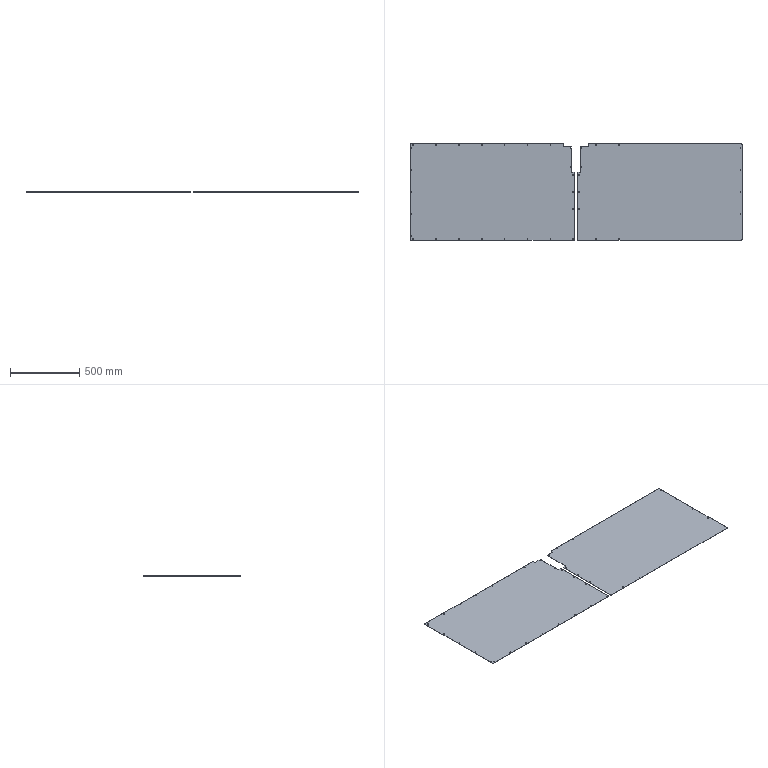Part | NX | features BREP 2 | 2 solids | 110 faces | box 2396 x 696 x 1.5 mm | volume 2460492 mm3 | cylinder 90 | plane 20 | commonest cylinder face diameters 5 x56 5.5 x20 6 x14